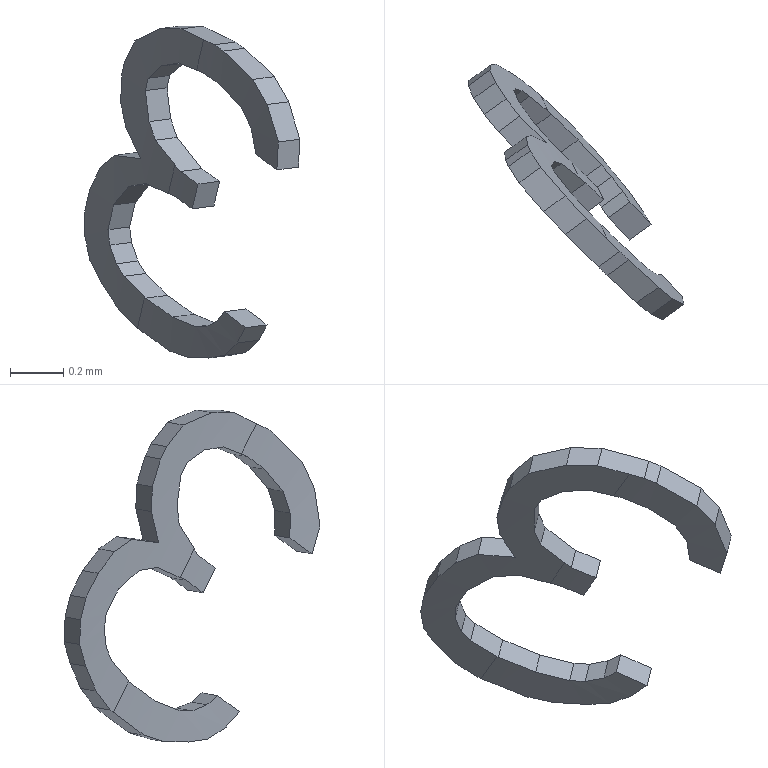Part | SolidWorks | features BaseBody 1 | 1 solid | 65 faces | box 0.8136 x 0.9655 x 1.252 mm | volume 0.03857 mm3 | plane 57 | cylinder 8 | commonest cylinder face diameters 16.8 x4 17 x4